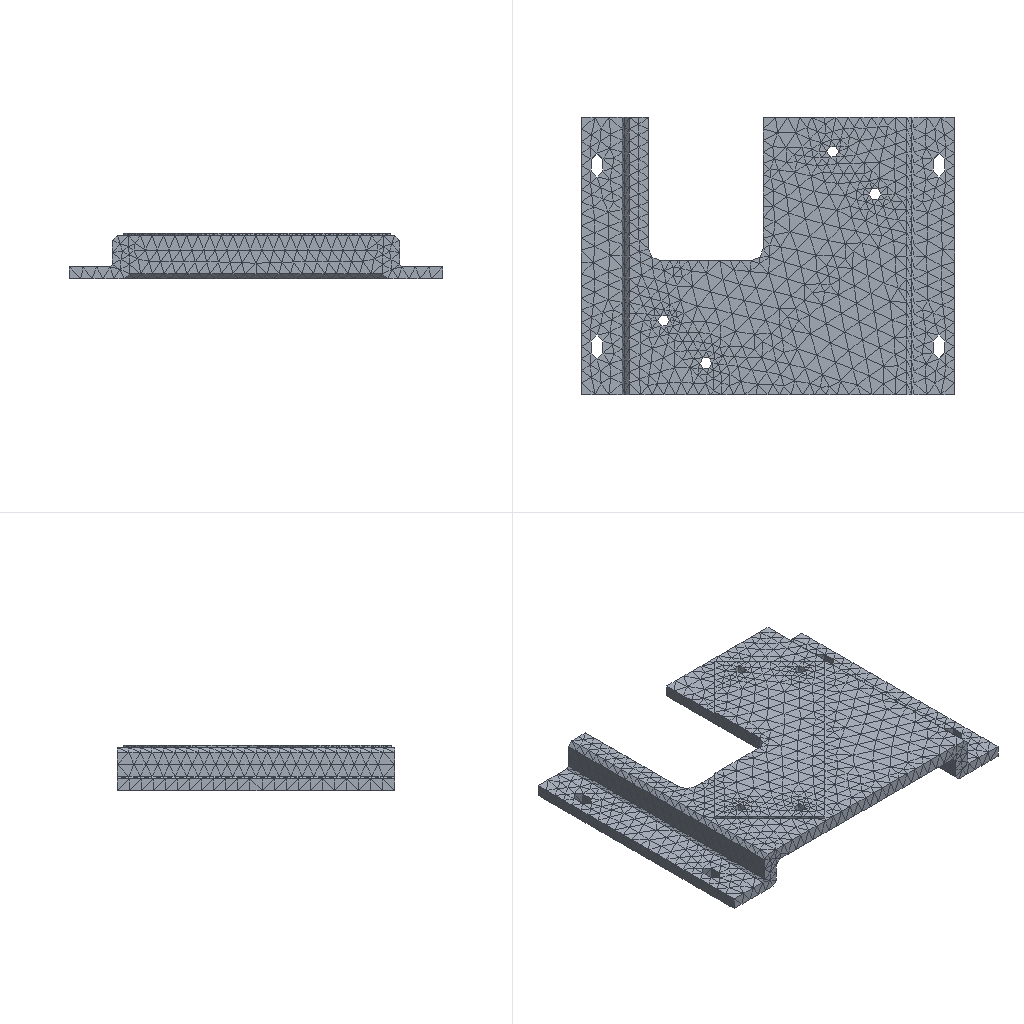Simulation study | nx simcenter
Set-up summary:
category,name,step,type,value,unit,region
solver,nx_nastran (Simcenter)
units,not stated in the deck,,not stated
analysis,deck,,static,static
analysis,solution,,SOL,101
load_step,SUBCASE 1,1,SUBCASE,SPC=1 LOAD=2
load_step,requested,,,1
mesh,nodes,,,12520
mesh,elements,,,6273
element_type,CTETRA,,solid,6273
load,nodal force total,,FX,0.0,model units
load,nodal force total,,FY,0.0,model units
load,nodal force total,,FZ,-999999.944,model units
load,load commands in deck,,count,666
bc,support commands in deck,,count,1079
analysis,NX solution 0,,Structural,Linear Statics - Single Constraint
check,setup vs results,,match,every grid point's frame and coordinates and every element id; grid points of CTETRA elements
Nastran input file, long lists of numbers shortened:
$*$$$$$$$$$$$$$$$$$$$$$$$$$$$$$$$$$$$$$$$$$$$$$$$$$$$$$$$$$$$$$$$$$
$*
$*                    NX v10.0.0.24 TRANSLATOR
$*                    FOR NX NASTRAN VERSION 10.0
$ (33 more lines like these left out)
ASSIGN OUTPUT2='127_sim1-solution_1.op2' UNIT=12
$*
$*$$$$$$$$$$$$$$$$$$$$$$$$$$$$$$$$$$$
$*
$* EXECUTIVE CONTROL
$*
$*$$$$$$$$$$$$$$$$$$$$$$$$$$$$$$$$$$$
$*
ID,NASTRAN,127_sim1-solution_1
SOL 101
CEND
$*
$*$$$$$$$$$$$$$$$$$$$$$$$$$$$$$$$$$$$
$*
$* CASE CONTROL
$*
$*$$$$$$$$$$$$$$$$$$$$$$$$$$$$$$$$$$$
$*
TITLE = Solution 1
ECHO = NONE
SPC = 1
OUTPUT
BCRESULTS(TRACTION,FORCE,PLOT) = ALL
DISPLACEMENT(PLOT) = ALL
ESE(PLOT) = ALL
FORCE(PLOT,CORNER) = ALL
OLOAD(PLOT) = ALL
SPCFORCES(PLOT) = ALL
STRAIN(PLOT,FIBER,CORNER) = ALL
STRESS(PLOT,CORNER) = ALL
$*  NX Step: Subcase - Static Loads 1
SUBCASE 1
LABEL = Subcase - Static Loads 1
LOAD = 2
$*
$*$$$$$$$$$$$$$$$$$$$$$$$$$$$$$$$$$$$
$*
$* BULK DATA
$*
$*$$$$$$$$$$$$$$$$$$$$$$$$$$$$$$$$$$$
$*
BEGIN BULK
$*
$* PARAM CARDS
$*
PARAM      K6ROT100.0000
PARAM     OIBULK     YES
PARAM    OMACHPR     YES
PARAM       POST      -2
PARAM    POSTEXT     YES
PARAM    UNITSYS   MN-MM
$*
$* GRID CARDS
$*
GRID*              12395               0-1.380000000E+02-1.160000000E+02+
*       -1.401000023E+01               0
GRID*              12396               0-1.380000000E+02-1.160000000E+02+
*       -9.010000229E+00               0
$ (25036 more lines like these left out)
$*
$* ELEMENT CARDS
$*
$*  NX Mesh Collector: Solid(1)
$*  NX Mesh: 3d_mesh(1)
CTETRA         1       1    9668    9650       1    9667   10032     141+
+            142   10033   10027     143
CTETRA         2       1   11741       1    9651    9673     144     145+
+           9951    9952     146    9953
$ (12542 more lines like these left out)
$*
$* PROPERTY CARDS
$*
$*  NX Property: PSOLID1
PSOLID         1       1       0                           SMECH
$*
$* MATERIAL CARDS
$*
$*  NX Material: Aluminum_2014
MAT1           17.3119+7        0.3300002.7940-62.1355-5
MATT1          1       1               2               3
TABLEM1        1                                                        +
+        20.00007.3119+7 21.11007.3119+7 23.89007.3119+7 37.78007.3119+7+
+        51.67007.3119+7 65.56007.2429+7 79.44007.2429+7 93.33007.1739+7+
+       107.22007.1049+7121.11007.0359+7135.00006.9670+7148.89006.8980+7+
+       162.78006.8290+7176.67006.6910+7190.56006.6221+7204.44006.4841+7+
+       218.33006.3461+7232.22006.1392+7246.11006.0012+7260.00005.8633+7+
+       273.89005.7253+7287.78005.5184+7301.67005.3804+7315.56005.1735+7+
+       329.44004.9665+7343.33004.7596+7357.22004.6216+7371.11004.4147+7+
+           ENDT
TABLEM1        2                                                        +
+        20.00000.330000 21.11000.330000    ENDT
TABLEM1        3                                                        +
+        20.00002.1600-5 93.33002.2500-5107.22002.2662-5121.11002.2824-5+
+       135.00002.2968-5148.89002.3130-5162.78002.3274-5176.67002.3418-5+
+       190.56002.3544-5204.44002.3688-5218.33002.3814-5232.22002.3958-5+
+       246.11002.4066-5260.00002.4192-5273.89002.4300-5287.78002.4408-5+
+       301.67002.4498-5315.56002.4606-5329.44002.4696-5343.33002.4786-5+
+       357.22002.4876-5371.11002.4984-5385.00002.5110-5398.89002.5254-5+
+       412.78002.5398-5426.67002.5560-5    ENDT
$*
$* LOAD AND CONSTRAINT CARDS
$*
$*  NX Load and Constraint: Fixed(1)
SPC            1    5813  123456  0.0000
SPC            1    5814  123456  0.0000
SPC            1    5815  123456  0.0000
SPC            1    5816  123456  0.0000
$ (1075 more lines like these left out)
$*  NX Load and Constraint: Force(1)
FORCE          2    7390       0795.9843  0.0000  0.0000-1.00000
FORCE          2    7391       0705.9189  0.0000  0.0000-1.00000
FORCE          2    7392       0713.2419  0.0000  0.0000-1.00000
FORCE          2    7393       0928.4338  0.0000  0.0000-1.00000
$ (662 more lines like these left out)
ENDDATA 8e18e02c
Results summary:
result,analysis,,,static
result,last_loadstep,,,1
result,primary field,,,displacements
result,max displacement,,,0.04994,model units
result,reaction total,,FX,0.07395,model units
result,reaction total,,FY,-0.07658,model units
result,reaction total,,FZ,1000000.062,model units
result,NX solution 0,,loadcases,1,mm